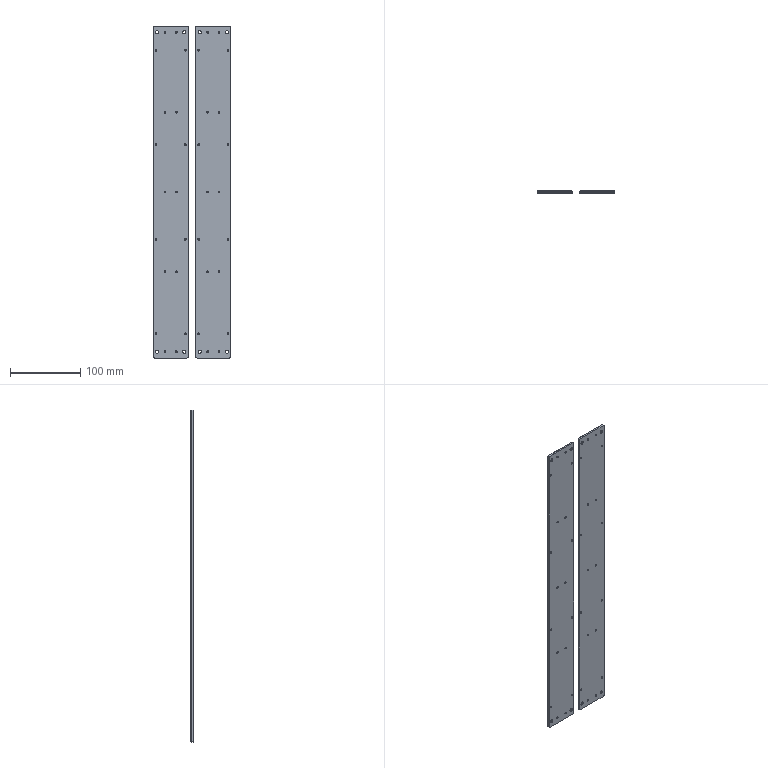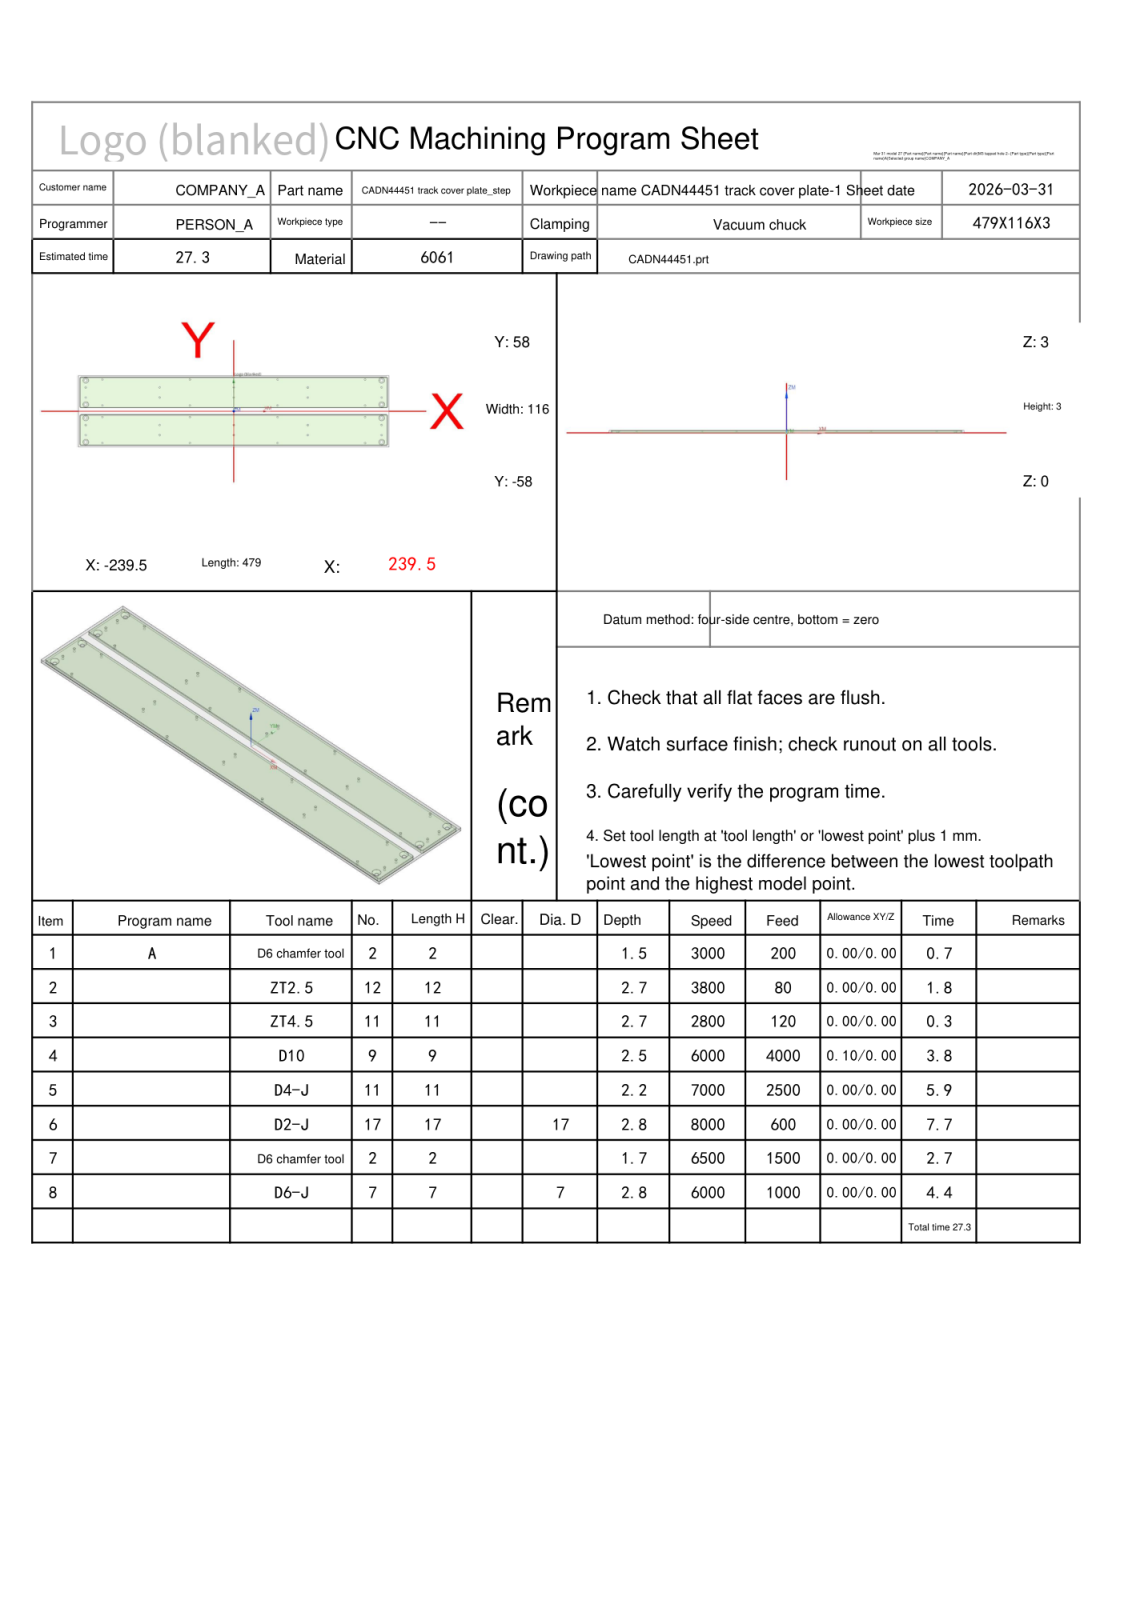NC program | NX | posted by the shop | part box 111 x 3 x 474 mm
Lines 1 to 278 of 17996:
%
O0001
(Machine time: 28.76 MIN)
(===Total Tool:6===)
(T2=D6 chamfer tool   D=6.   R=0.   D-  H02 Z=1.25  )
(T12=ZT2.5  D=2.5  DR_a=118 D-  H12 Z=0.3   )
(T11=ZT4.5  D=4.5  DR_a=118 D-  H11 Z=0.3   )
(T9=D10     D=10.  R=0.   D-  H09 Z=0.5   )
(T17=D2-J   D=2.   R=0.   D17 H17 Z=0.15  )
(T7=D6-J    D=6.   R=0.   D7  H07 Z=0.2   )
G80 G90 G17 G49 G40
G91 G28 Z0
M01
N1 T02 M06
(D6 chamfer tool  D=6. R=0. H=02 ce=0.00 di=0.00)
G00 G90 G54 X228. Y50. M03 S3000
G43 H02 Z23.
M08
G98 G81 X228. Y50. Z1.5 R4. F200.
Y11.
Y-11.
Y-50.
X-228.
Y-11.
Y11.
Y50.
G80
G00 Z23.
G00 G90 X202.5 Y51.5 M03 S3000
Z23.
G98 G81 X202.5 Y51.5 Z2. R4. F200.
X228. Y38.6
Y22.4
X202.5 Y9.5
Y-9.5
X228. Y-22.4
Y-38.6
X202.5 Y-51.5
X114. Y-38.6
Y-22.4
Y22.4
Y38.6
X67.5 Y51.5
Y9.5
Y-9.5
Y-51.5
X0.0 Y-38.6
Y-22.4
Y22.4
Y38.6
X-67.5 Y51.5
Y9.5
Y-9.5
Y-51.5
X-114. Y-38.6
Y-22.4
Y22.4
Y38.6
X-202.5 Y51.5
X-228. Y38.6
Y22.4
X-202.5 Y9.5
Y-9.5
X-228. Y-22.4
Y-38.6
X-202.5 Y-51.5
G80
G00 Z23.
G91 G28 Z0.0
M05
M09
G91 G28 Z0.0
M01
N2 T12 M06
(ZT2.5 D=2.5 DR_a=118 H=12)
G00 G90 G54 X202.5 Y51.5 M03 S3800
G43 H12 Z23.
M08
G98 G83 X202.5 Y51.5 Z.3 R4. F80. Q1.5
X228. Y38.6
Y22.4
X202.5 Y9.5
Y-9.5
X228. Y-22.4
Y-38.6
X202.5 Y-51.5
X114. Y-38.6
Y-22.4
Y22.4
Y38.6
X67.5 Y51.5
Y9.5
Y-9.5
Y-51.5
X0.0 Y-38.6
Y-22.4
Y22.4
Y38.6
X-67.5 Y51.5
Y9.5
Y-9.5
Y-51.5
X-114. Y-38.6
Y-22.4
Y22.4
Y38.6
X-202.5 Y51.5
X-228. Y38.6
Y22.4
X-202.5 Y9.5
Y-9.5
X-228. Y-22.4
Y-38.6
X-202.5 Y-51.5
G80
G00 Z23.
G91 G28 Z0.0
M05
M09
G91 G28 Z0.0
M01
N3 T11 M06
(ZT4.5 D=4.5 DR_a=118 H=11)
G00 G90 G54 X228. Y50. M03 S2800
G43 H11 Z23.
M08
G98 G83 X228. Y50. Z.3 R4. F120. Q1.5
Y11.
Y-11.
Y-50.
X-228.
Y-11.
Y11.
Y50.
G80
G00 Z23.
G91 G28 Z0.0
M05
M09
G91 G28 Z0.0
M01
N4 T09 M06
(D10  D=10. R=0. H=09 ce=0.10 di=0.00)
G00 G90 G54 X0.0 Y60.6 M03 S6000
G43 H09 Z23.
M08
Z3.5
G01 X235. Z3.391 F4000.
G02 X242.1 Y53.5 Z3.386 I0.0 J-7.1
G01 Y7.5 Z3.364
G02 X235. Y.4 Z3.359 I-7.1 J0.0
G01 X-235. Z3.141
G02 X-242.1 Y7.5 Z3.136 I0.0 J7.1
G01 Y53.5 Z3.114
G02 X-235. Y60.6 Z3.109 I7.1 J0.0
G01 X235. Z2.891
G02 X242.1 Y53.5 Z2.886 I0.0 J-7.1
G01 Y7.5 Z2.864
G02 X235. Y.4 Z2.859 I-7.1 J0.0
G01 X-235. Z2.641
G02 X-242.1 Y7.5 Z2.636 I0.0 J7.1
G01 Y53.5 Z2.614
G02 X-235. Y60.6 Z2.609 I7.1 J0.0
G01 X235. Z2.391
G02 X242.1 Y53.5 Z2.386 I0.0 J-7.1
G01 Y7.5 Z2.364
G02 X235. Y.4 Z2.359 I-7.1 J0.0
G01 X-235. Z2.141
G02 X-242.1 Y7.5 Z2.136 I0.0 J7.1
G01 Y53.5 Z2.114
G02 X-235. Y60.6 Z2.109 I7.1 J0.0
G01 X235. Z1.891
G02 X242.1 Y53.5 Z1.886 I0.0 J-7.1
G01 Y7.5 Z1.864
G02 X235. Y.4 Z1.859 I-7.1 J0.0
G01 X-235. Z1.641
G02 X-242.1 Y7.5 Z1.636 I0.0 J7.1
G01 Y53.5 Z1.614
G02 X-235. Y60.6 Z1.609 I7.1 J0.0
G01 X235. Z1.391
G02 X242.1 Y53.5 Z1.386 I0.0 J-7.1
G01 Y7.5 Z1.364
G02 X235. Y.4 Z1.359 I-7.1 J0.0
G01 X-235. Z1.141
G02 X-242.1 Y7.5 Z1.136 I0.0 J7.1
G01 Y53.5 Z1.114
G02 X-235. Y60.6 Z1.109 I7.1 J0.0
G01 X235. Z.891
G02 X242.1 Y53.5 Z.886 I0.0 J-7.1
G01 Y7.5 Z.864
G02 X235. Y.4 Z.859 I-7.1 J0.0
G01 X-235. Z.641
G02 X-242.1 Y7.5 Z.636 I0.0 J7.1
G01 Y53.5 Z.614
G02 X-235. Y60.6 Z.609 I7.1 J0.0
G01 X0.0 Z.5
X235.
G02 X242.1 Y53.5 I0.0 J-7.1
G01 Y7.5
G02 X235. Y.4 I-7.1 J0.0
G01 X-235.
G02 X-242.1 Y7.5 I0.0 J7.1
G01 Y53.5
G02 X-235. Y60.6 I7.1 J0.0
G01 X0.0
X.5
Z1.5
G00 Z23.
X0.0 Y-60.6
Z3.5
G01 X-235. Z3.391
G02 X-242.1 Y-53.5 Z3.386 I0.0 J7.1
G01 Y-7.5 Z3.364
G02 X-235. Y-.4 Z3.359 I7.1 J0.0
G01 X235. Z3.141
G02 X242.1 Y-7.5 Z3.136 I0.0 J-7.1
G01 Y-53.5 Z3.114
G02 X235. Y-60.6 Z3.109 I-7.1 J0.0
G01 X-235. Z2.891
G02 X-242.1 Y-53.5 Z2.886 I0.0 J7.1
G01 Y-7.5 Z2.864
G02 X-235. Y-.4 Z2.859 I7.1 J0.0
G01 X235. Z2.641
G02 X242.1 Y-7.5 Z2.636 I0.0 J-7.1
G01 Y-53.5 Z2.614
G02 X235. Y-60.6 Z2.609 I-7.1 J0.0
G01 X-235. Z2.391
G02 X-242.1 Y-53.5 Z2.386 I0.0 J7.1
G01 Y-7.5 Z2.364
G02 X-235. Y-.4 Z2.359 I7.1 J0.0
G01 X235. Z2.141
G02 X242.1 Y-7.5 Z2.136 I0.0 J-7.1
G01 Y-53.5 Z2.114
G02 X235. Y-60.6 Z2.109 I-7.1 J0.0
G01 X-235. Z1.891
G02 X-242.1 Y-53.5 Z1.886 I0.0 J7.1
G01 Y-7.5 Z1.864
G02 X-235. Y-.4 Z1.859 I7.1 J0.0
G01 X235. Z1.641
G02 X242.1 Y-7.5 Z1.636 I0.0 J-7.1
G01 Y-53.5 Z1.614
G02 X235. Y-60.6 Z1.609 I-7.1 J0.0
G01 X-235. Z1.391
G02 X-242.1 Y-53.5 Z1.386 I0.0 J7.1
G01 Y-7.5 Z1.364
G02 X-235. Y-.4 Z1.359 I7.1 J0.0
G01 X235. Z1.141
G02 X242.1 Y-7.5 Z1.136 I0.0 J-7.1
G01 Y-53.5 Z1.114
G02 X235. Y-60.6 Z1.109 I-7.1 J0.0
G01 X-235. Z.891
G02 X-242.1 Y-53.5 Z.886 I0.0 J7.1
G01 Y-7.5 Z.864
G02 X-235. Y-.4 Z.859 I7.1 J0.0
G01 X235. Z.641
G02 X242.1 Y-7.5 Z.636 I0.0 J-7.1
G01 Y-53.5 Z.614
G02 X235. Y-60.6 Z.609 I-7.1 J0.0
G01 X0.0 Z.5
X-235.
G02 X-242.1 Y-53.5 I0.0 J7.1
G01 Y-7.5
G02 X-235. Y-.4 I7.1 J0.0
G01 X235.
G02 X242.1 Y-7.5 I0.0 J-7.1
G01 Y-53.5
G02 X235. Y-60.6 I-7.1 J0.0
G01 X0.0
X-.5
Z1.5
G00 Z23.
G91 G28 Z0.0
M05
M09
G91 G28 Z0.0
M01